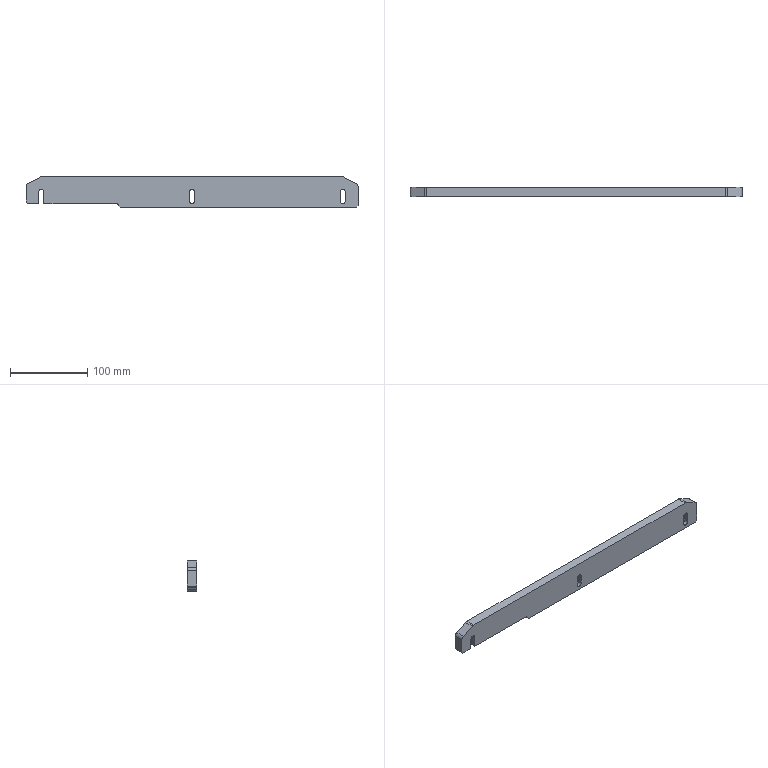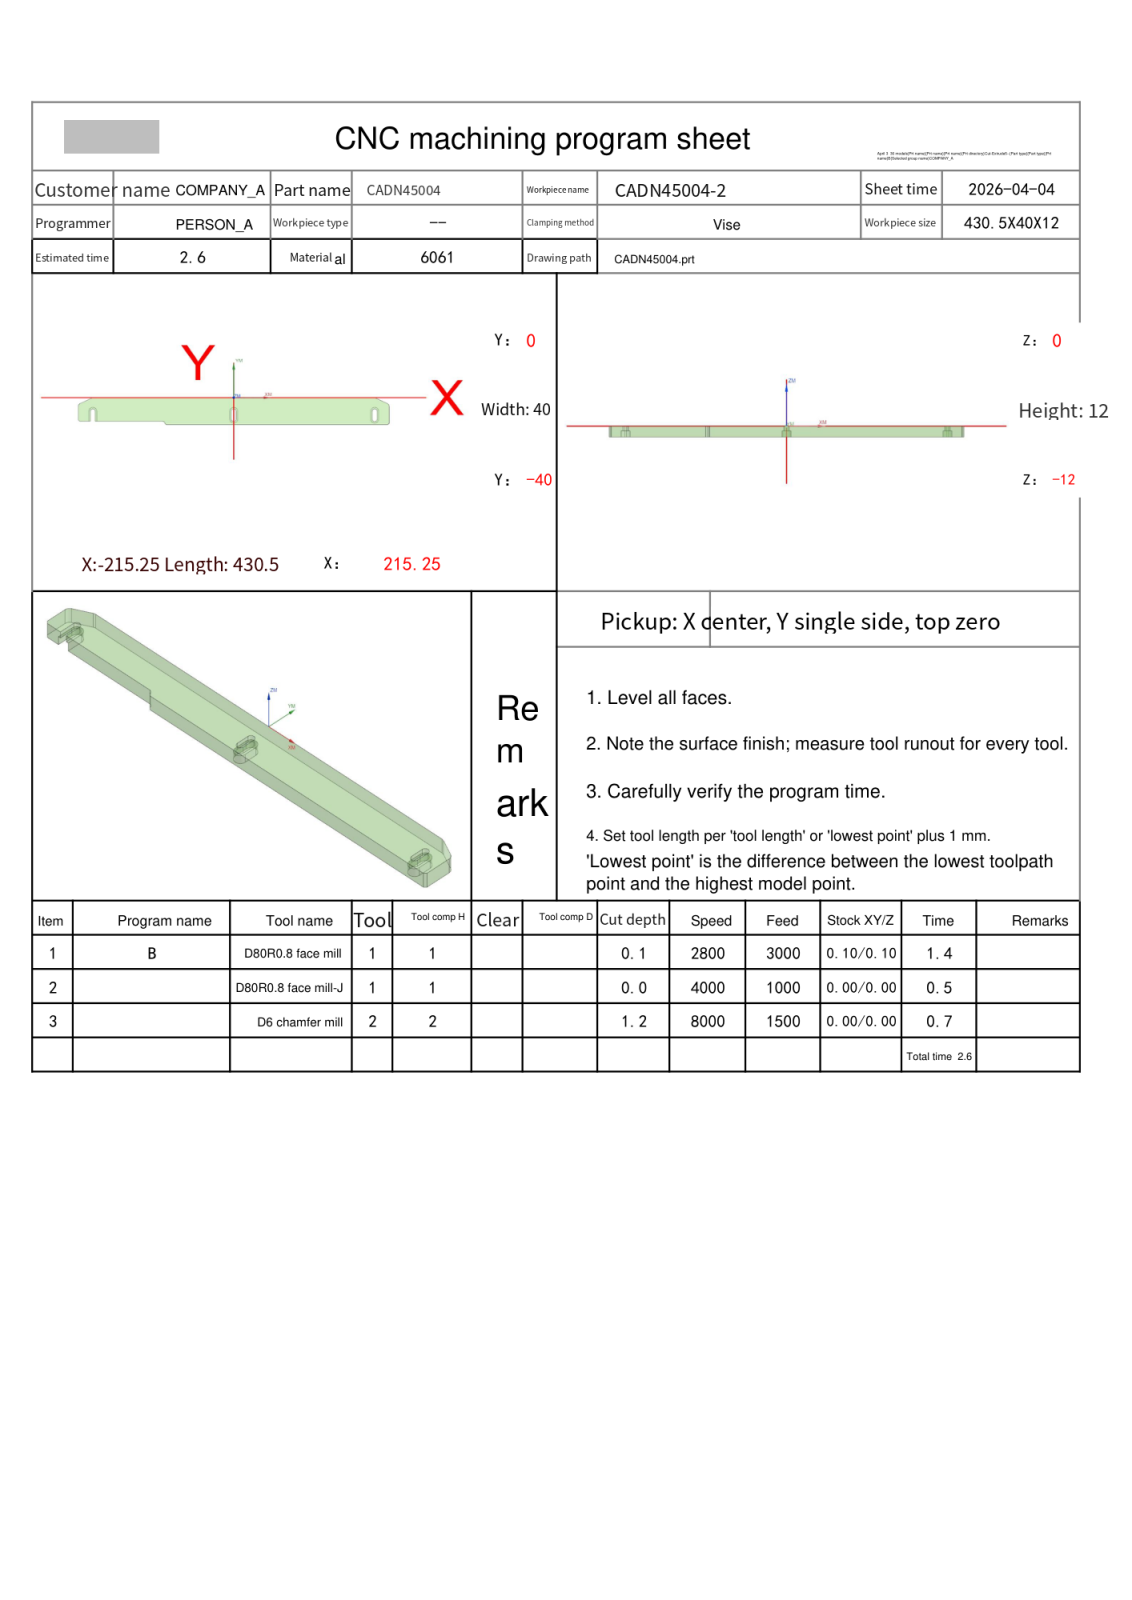NC program | NX | posted by the shop | part box 430.5 x 12 x 40 mm
Whole program:
%
O0001
(Machine time: 3.21 MIN)
(===Total Tool:2===)
(T1=D80R0.8 face mill D=80.  R=0.8  D-  H01 Z=0.    )
(T2=D6 chamfer mill   D=6.   R=0.   D-  H02 Z=-1.2  )
G80 G90 G17 G49 G40
G91 G28 Z0
M01
N1 T01 M06
(D80R0.8 face mill  D=80. R=0.8 H=01 ce=0.10 di=0.10)
G00 G90 G54 X267.347 Y-16.901 M03 S2800
G43 H01 Z50.
M08
Z4.517
G01 Z2.517 F3000.
X255.347 Y-17.045
X-255.347 Y-23.186
X-267.347 Y-23.33
Z4.517
G00 X267.347 Y-16.901
Z4.033
G01 Z2.033
X255.347 Y-17.045
X-255.347 Y-23.186
X-267.347 Y-23.33
Z4.033
G00 X267.347 Y-16.901
Z3.55
G01 Z1.55
X255.347 Y-17.045
X-255.347 Y-23.186
X-267.347 Y-23.33
Z3.55
G00 X267.347 Y-16.901
Z3.067
G01 Z1.067
X255.347 Y-17.045
X-255.347 Y-23.186
X-267.347 Y-23.33
Z3.067
G00 Z50.
X267.347 Y-16.901
Z2.583
G01 Z.583
X255.347 Y-17.045
X-255.347 Y-23.186
X-267.347 Y-23.33
Z2.583
G00 Z50.
X267.347 Y-16.901
Z2.1
G01 Z.1
X255.347 Y-17.045
X-255.347 Y-23.186
X-267.347 Y-23.33
Z2.1
G00 Z50.
G91 G28 Z0.0
M05
M09
G91 G28 Z0.0
M01
N2 T01 M06
(D80R0.8 face mill-J  D=80. R=0.8 H=01 ce=0.00 di=0.00)
G00 G90 G54 X267.249 Y-16.898 M03 S4000
G43 H01 Z50.
M08
Z2.
G01 Z0.0 F1000.
X255.249 Y-17.043
X-255.249 Y-23.188
X-267.249 Y-23.332
Z2.
G00 Z50.
G91 G28 Z0.0
M05
M09
G91 G28 Z0.0
M01
N3 T02 M06
(D6 chamfer mill  D=6. R=0. H=02 ce=0.00 di=0.00)
G00 G90 G54 X-.386 Y1.127 M03 S8000
G43 H02 Z50.
M08
Z.272
G01 Z-1.2 F1350.
G03 X-.1 Y.927 I1.286 J1.532
G01 X-.054 Y.897
X0.0 Y.9
X194.07 F1500.
X194.752 Y.86
X195.425 Y.742
X196.08 Y.547
X196.708 Y.277
X212.889 Y-7.813
G02 X216.15 Y-13.09 I-2.639 J-5.277
G01 Y-38.
X216.119 Y-38.233
X216.029 Y-38.45
X215.886 Y-38.636
X213.886 Y-40.636
X213.7 Y-40.779
X213.483 Y-40.869
X213.25 Y-40.9
X-93.25
X-93.483 Y-40.869
X-93.7 Y-40.779
X-93.886 Y-40.636
X-95.886 Y-38.636
X-96.029 Y-38.45
X-96.119 Y-38.233
X-96.15 Y-38.
G03 X-98.25 Y-35.9 I-2.1 J0.0
G01 X-191.95
G02 X-192.85 Y-35. I0.0 J.9
G01 Y-20.
G03 X-195.25 Y-17.6 I-2.4 J0.0
X-197.65 Y-20. I0.0 J-2.4
G01 Y-35.
G02 X-198.55 Y-35.9 I-.9 J0.0
G01 X-213.25
X-213.483 Y-35.869
X-213.7 Y-35.779
X-213.886 Y-35.636
X-215.886 Y-33.636
X-216.029 Y-33.45
X-216.119 Y-33.233
X-216.15 Y-33.
Y-13.09
G02 X-212.889 Y-7.813 I5.9 J0.0
G01 X-196.708 Y.277
X-196.08 Y.547
X-195.425 Y.742
X-194.752 Y.86
X-194.07 Y.9
X0.0
X.054 Y.897
X.1 Y.927
G03 X.386 Y1.127 I-1. J1.732
G01 Z.272
G00 Z10.
X2.173 Y-26.386
Z.272
G01 Z-1.2 F1350.
G03 X2.373 Y-26.1 I-1.532 J1.286
G01 X2.403 Y-26.054
X2.4 Y-26.
Y-20. F1500.
G03 X0.0 Y-17.6 I-2.4 J0.0
X-2.4 Y-20. I0.0 J-2.4
G01 Y-32.
G03 X0.0 Y-34.4 I2.4 J0.0
X2.4 Y-32. I0.0 J2.4
G01 Y-26.
X2.403 Y-25.946
X2.373 Y-25.9
G03 X2.173 Y-25.614 I-1.732 J-1.
G01 Z.272
G00 Z10.
X193.077
Z.272
G01 Z-1.2 F1350.
G03 X192.877 Y-25.9 I1.532 J-1.286
G01 X192.847 Y-25.946
X192.85 Y-26.
Y-32. F1500.
G03 X195.25 Y-34.4 I2.4 J0.0
X197.65 Y-32. I0.0 J2.4
G01 Y-20.
G03 X195.25 Y-17.6 I-2.4 J0.0
X192.85 Y-20. I0.0 J-2.4
G01 Y-26.
X192.847 Y-26.054
X192.877 Y-26.1
G03 X193.077 Y-26.386 I1.732 J1.
G01 Z.272
G00 Z50.
M05
M09
G91 G28 Z0.0
G91 G28 Y0.0
M30
%